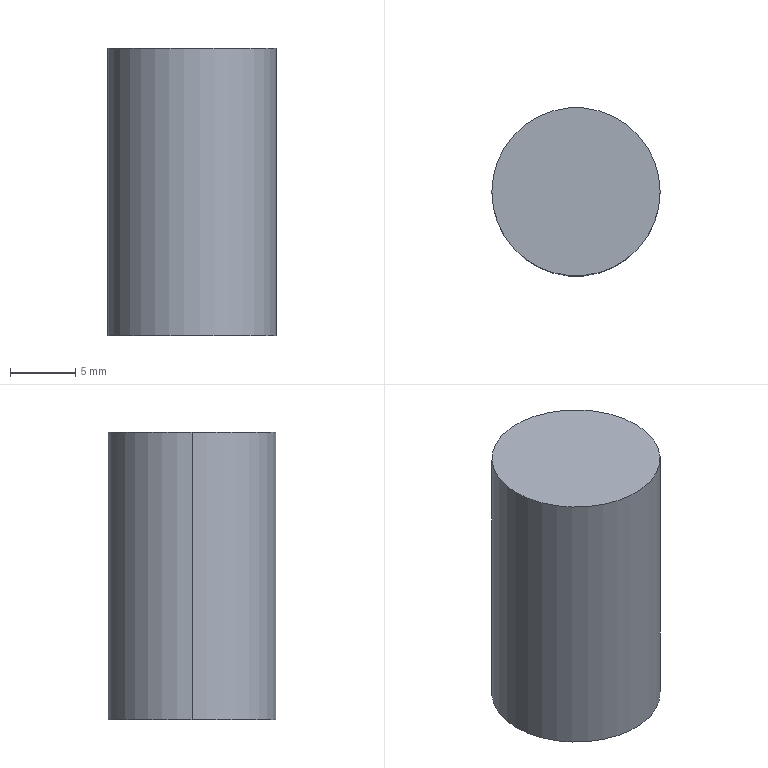Part | STEP file | 4-20.sldasm-Part-338 | 1 solid | 4 faces | box 12.862 x 12.862 x 22 mm | volume 2859 mm3 | cylinder 2 | plane 2 | commonest cylinder face diameters 12.862 x2
STEP:
#1=CARTESIAN_POINT('',(2.569,70.,115.));
#2=VERTEX_POINT('',#1);
#3=CARTESIAN_POINT('',(15.431,70.,115.));
#4=VERTEX_POINT('',#3);
#5=CARTESIAN_POINT('',(9.,70.,115.));
#6=DIRECTION('',(0.,0.,-1.));
#7=DIRECTION('',(-1.,0.,0.));
#8=AXIS2_PLACEMENT_3D('',#5,#6,#7);
#9=CIRCLE('',#8,6.431);
#10=EDGE_CURVE('',#2,#4,#9,.T.);
#11=ORIENTED_EDGE('',*,*,#10,.T.);
#12=CARTESIAN_POINT('',(15.431,70.,93.));
#13=VERTEX_POINT('',#12);
#14=CARTESIAN_POINT('',(15.431,70.,115.));
#15=DIRECTION('',(0.,0.,-1.));
#16=VECTOR('',#15,1000.);
#17=LINE('',#14,#16);
#18=EDGE_CURVE('',#4,#13,#17,.T.);
#19=ORIENTED_EDGE('',*,*,#18,.T.);
#20=CARTESIAN_POINT('',(2.569,70.,93.));
#21=VERTEX_POINT('',#20);
#22=CARTESIAN_POINT('',(9.,70.,93.));
#23=DIRECTION('',(0.,0.,-1.));
#24=DIRECTION('',(-1.,0.,0.));
#25=AXIS2_PLACEMENT_3D('',#22,#23,#24);
#26=CIRCLE('',#25,6.431);
#27=EDGE_CURVE('',#21,#13,#26,.T.);
#28=ORIENTED_EDGE('',*,*,#27,.F.);
#29=CARTESIAN_POINT('',(2.569,70.,115.));
#30=DIRECTION('',(0.,0.,-1.));
#31=VECTOR('',#30,1000.);
#32=LINE('',#29,#31);
#33=EDGE_CURVE('',#2,#21,#32,.T.);
#34=ORIENTED_EDGE('',*,*,#33,.F.);
#35=EDGE_LOOP('',(#11,#19,#28,#34));
#36=FACE_OUTER_BOUND('',#35,.T.);
#37=CARTESIAN_POINT('',(9.,70.,115.));
#38=DIRECTION('',(0.,0.,-1.));
#39=DIRECTION('',(-1.,0.,0.));
#40=AXIS2_PLACEMENT_3D('',#37,#38,#39);
#41=CYLINDRICAL_SURFACE('',#40,6.431);
#42=ADVANCED_FACE('',(#36),#41,.T.);
#43=ORIENTED_EDGE('',*,*,#18,.F.);
#44=CARTESIAN_POINT('',(9.,70.,115.));
#45=DIRECTION('',(0.,0.,-1.));
#46=DIRECTION('',(-1.,0.,0.));
#47=AXIS2_PLACEMENT_3D('',#44,#45,#46);
#48=CIRCLE('',#47,6.431);
#49=EDGE_CURVE('',#4,#2,#48,.T.);
#50=ORIENTED_EDGE('',*,*,#49,.T.);
#51=ORIENTED_EDGE('',*,*,#33,.T.);
#52=CARTESIAN_POINT('',(9.,70.,93.));
#53=DIRECTION('',(0.,0.,-1.));
#54=DIRECTION('',(-1.,0.,0.));
#55=AXIS2_PLACEMENT_3D('',#52,#53,#54);
#56=CIRCLE('',#55,6.431);
#57=EDGE_CURVE('',#13,#21,#56,.T.);
#58=ORIENTED_EDGE('',*,*,#57,.F.);
#59=EDGE_LOOP('',(#43,#50,#51,#58));
#60=FACE_OUTER_BOUND('',#59,.T.);
#61=CARTESIAN_POINT('',(9.,70.,115.));
#62=DIRECTION('',(0.,0.,-1.));
#63=DIRECTION('',(-1.,0.,0.));
#64=AXIS2_PLACEMENT_3D('',#61,#62,#63);
#65=CYLINDRICAL_SURFACE('',#64,6.431);
#66=ADVANCED_FACE('',(#60),#65,.T.);
#67=ORIENTED_EDGE('',*,*,#10,.F.);
#68=ORIENTED_EDGE('',*,*,#49,.F.);
#69=EDGE_LOOP('',(#67,#68));
#70=FACE_OUTER_BOUND('',#69,.T.);
#71=CARTESIAN_POINT('',(9.,-250.,115.));
#72=DIRECTION('',(0.,0.,-1.));
#73=DIRECTION('',(-1.,0.,0.));
#74=AXIS2_PLACEMENT_3D('',#71,#72,#73);
#75=PLANE('',#74);
#76=ADVANCED_FACE('',(#70),#75,.F.);
#77=ORIENTED_EDGE('',*,*,#27,.T.);
#78=ORIENTED_EDGE('',*,*,#57,.T.);
#79=EDGE_LOOP('',(#77,#78));
#80=FACE_OUTER_BOUND('',#79,.T.);
#81=CARTESIAN_POINT('',(9.,-250.,93.));
#82=DIRECTION('',(0.,0.,-1.));
#83=DIRECTION('',(-1.,0.,0.));
#84=AXIS2_PLACEMENT_3D('',#81,#82,#83);
#85=PLANE('',#84);
#86=ADVANCED_FACE('',(#80),#85,.T.);
#87=CLOSED_SHELL('',(#42,#66,#76,#86));
#88=MANIFOLD_SOLID_BREP('',#87);
#89=CARTESIAN_POINT('',(0.,0.,0.));
#90=DIRECTION('',(0.,0.,1.));
#91=DIRECTION('',(1.,0.,0.));
#92=AXIS2_PLACEMENT_3D('',#89,#90,#91);
#93=(LENGTH_UNIT()NAMED_UNIT(*)SI_UNIT(.MILLI.,.METRE.));
#94=UNCERTAINTY_MEASURE_WITH_UNIT(LENGTH_MEASURE(0.00001),#93,'','');
#95=(NAMED_UNIT(*)PLANE_ANGLE_UNIT()SI_UNIT($,.RADIAN.));
#96=(NAMED_UNIT(*)SI_UNIT($,.STERADIAN.)SOLID_ANGLE_UNIT());
#97=(GEOMETRIC_REPRESENTATION_CONTEXT(3)GLOBAL_UNCERTAINTY_ASSIGNED_CONTEXT((#94))GLOBAL_UNIT_ASSIGNED_CONTEXT((#93,#95,#96))REPRESENTATION_CONTEXT('',''));
#98=ADVANCED_BREP_SHAPE_REPRESENTATION('',(#88,#92),#97);